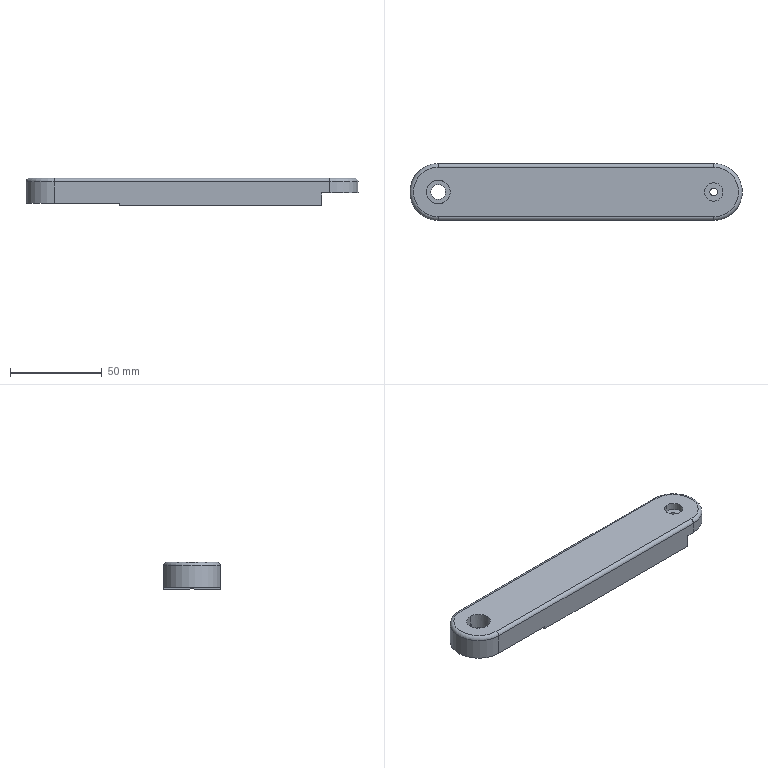Part | 1 solid | 100 faces | box 181 x 31 x 15 mm | volume 68722 mm3 | cylinder 48 | plane 26 | cone 24 | torus 2 | commonest cylinder face diameters 1.5 x8 1.6 x8 2 x8 2.05 x4 8.6 x4 0.4 x2